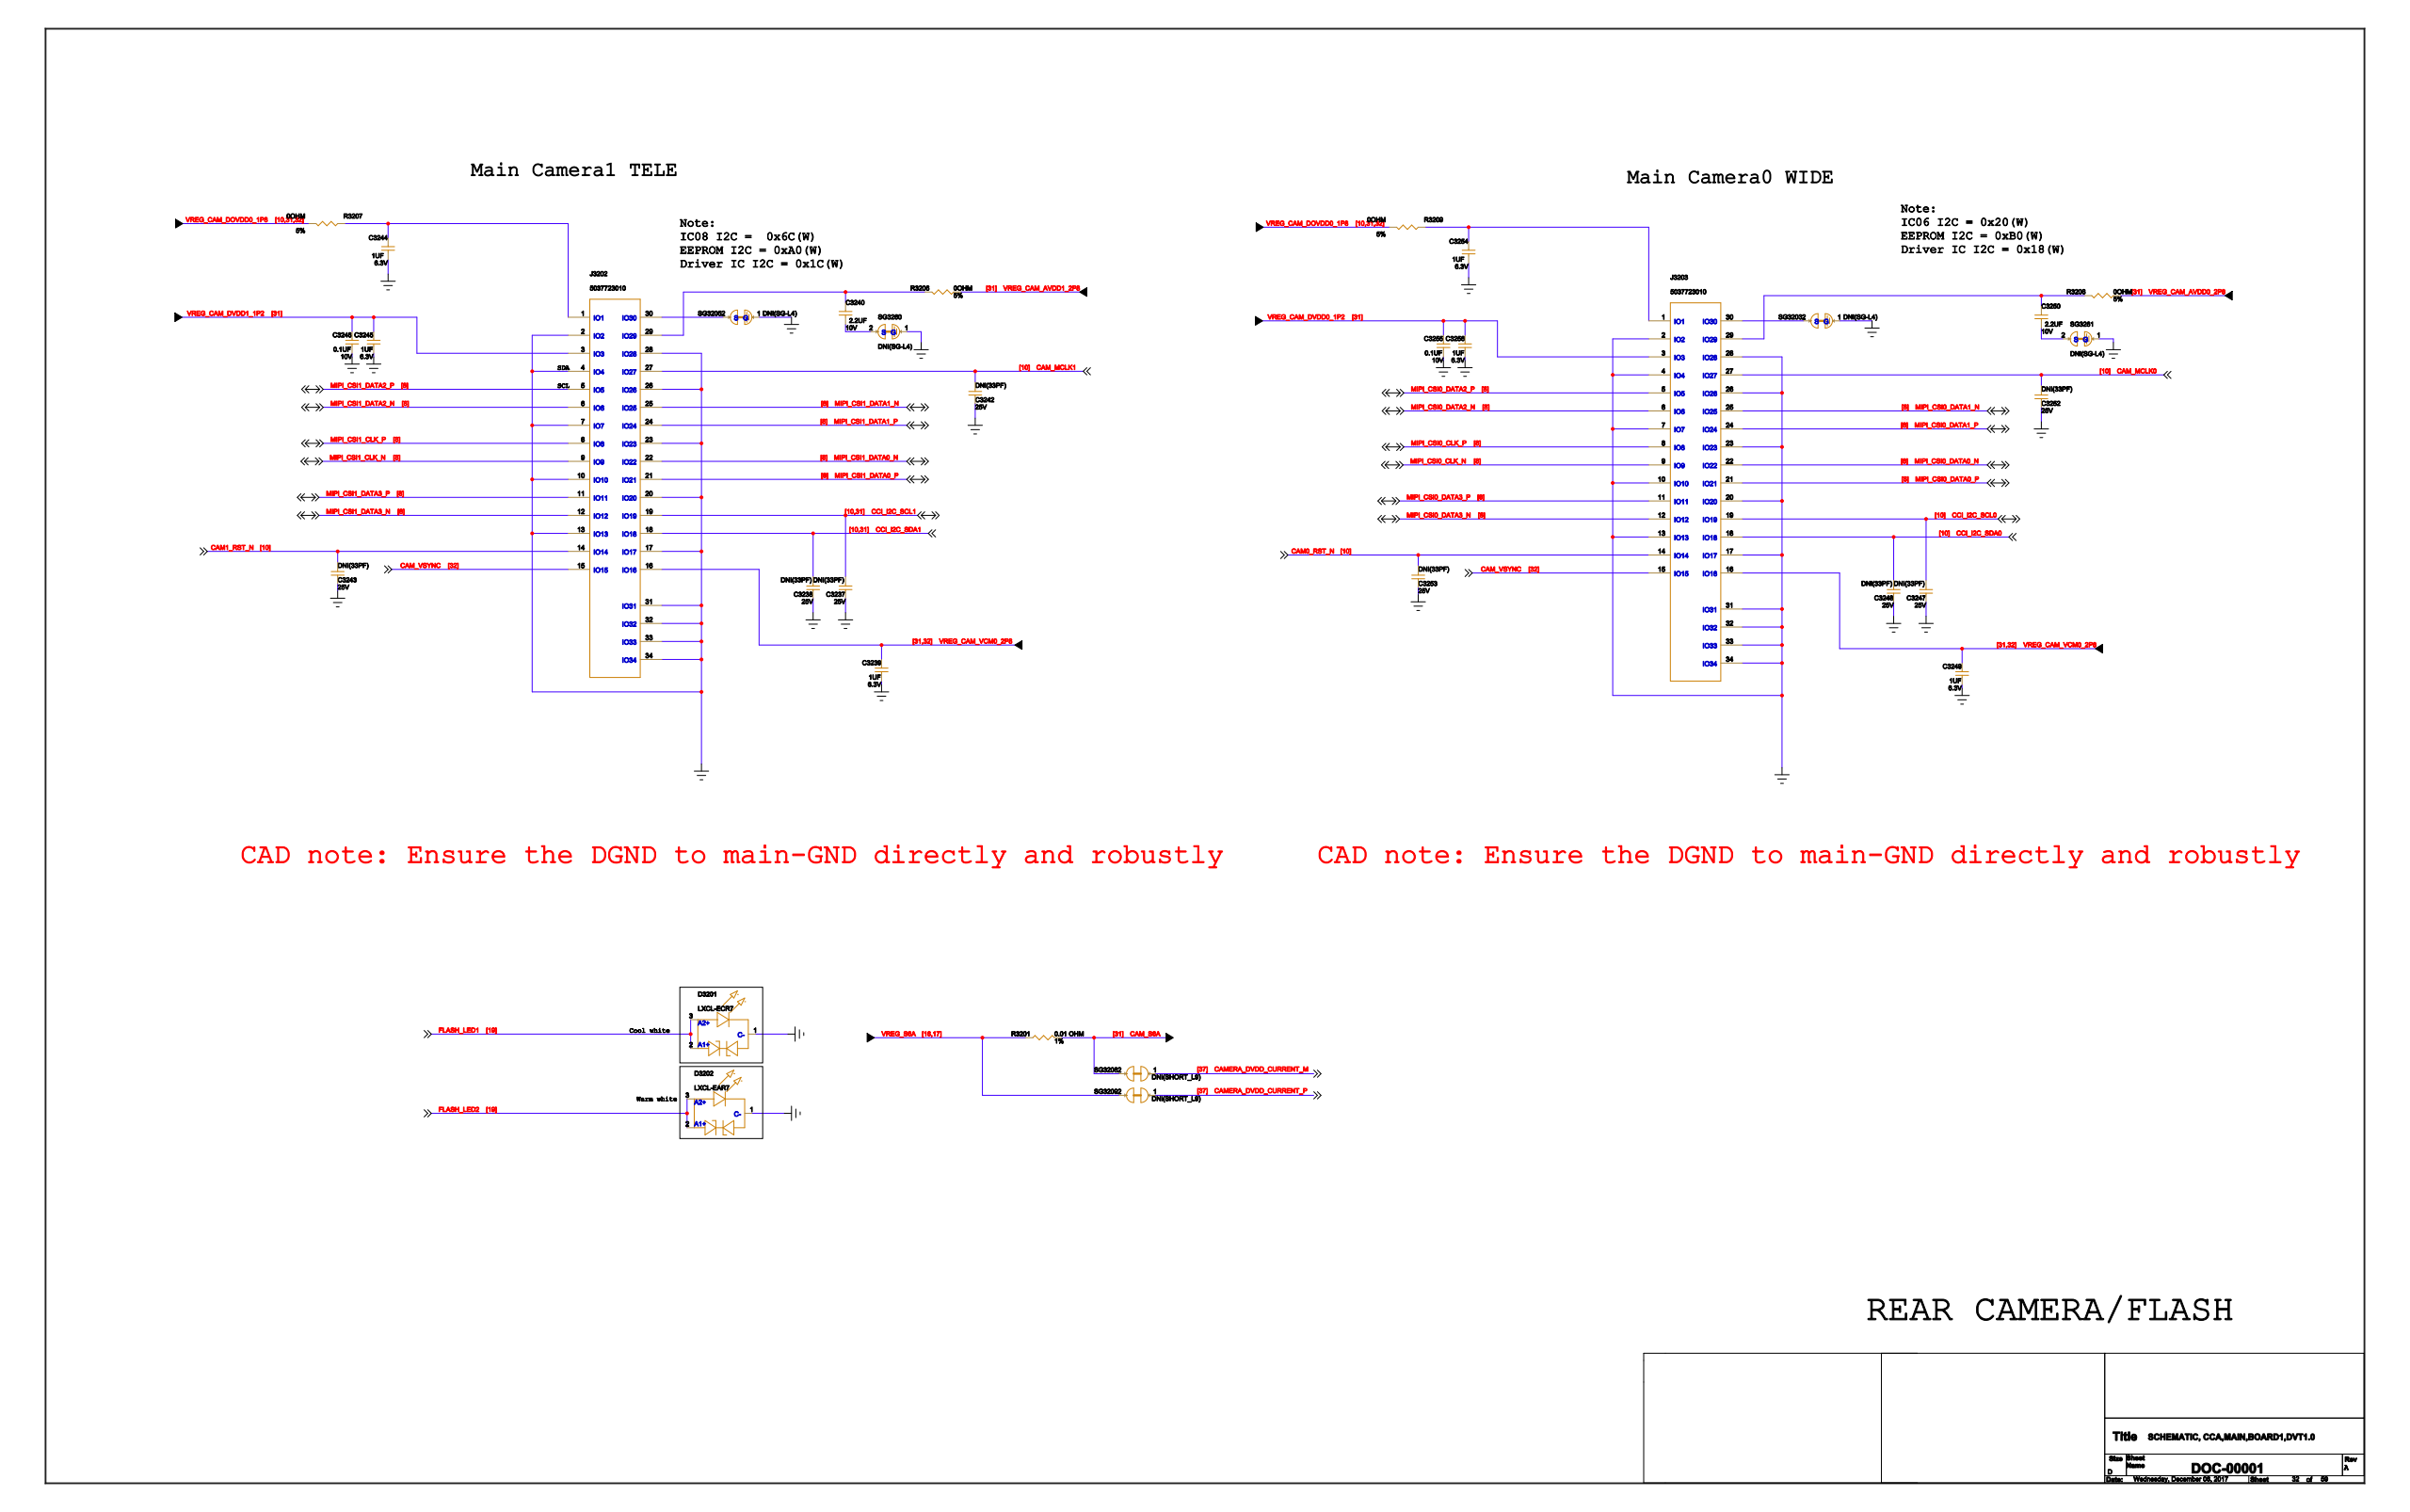Circuit board | KiCad | 1657 parts | 1365 nets | one sheet of the schematic
Parts on this sheet (reference | value | footprint):
C3237
C3238
C3239
C3240
C3242
C3243
C3244
C3245
C3246
C3247
C3248
C3249
C3250
C3252
C3253
C3254
C3255
C3256
D3202
J3202
J3203
R3201
R3206
R3207
R3208
R3209
SG3203
SG3205
SG3208
SG3209
SG3260
SG3261
Nets of these parts (net: part-pin ...):
GND: C3237-1 C3238-1 C3239-2 C3242-1 C3243-1 C3244-2 C3245-2 C3246-2 C3247-1 C3248-1 C3249-2 C3252-1 C3253-1 C3254-2 C3255-2 C3256-2 D3202-1 SG3203-1 SG3205-1 SG3260-1 SG3261-1 J3202-2 J3202-4 J3202-7 J3202-10 J3202-13 J3202-17 J3202-20 J3202-23 J3202-26 J3202-28 J3202-31 J3202-32 J3202-33 J3202-34 J3203-2 J3203-4 J3203-7 J3203-10 J3203-13 J3203-17 J3203-20 J3203-23 J3203-26 J3203-28 J3203-31 J3203-32 J3203-33 J3203-34
N21587930: SG3205-2 J3202-30
_CAM_DVDD1_1P2: C3245-1 C3246-1 J3202-3
N22393502: C3240-2 SG3260-2
_CAM_AVDD0_2P8: R3208-1
N21587625: C3250-1 R3208-2 J3203-29
N21587642: C3250-2 SG3261-2
CAM_DOVDD0_1P8: R3207-1 R3209-1
CCI_I2C_SCL0: C3247-2 J3203-19
_CAM_AVDD1_2P8: R3206-1
DVDD_CURRENT_P: SG3209-1
VREG_S6A: R3201-2 SG3209-2
CCI_I2C_SDA1: C3238-2 J3202-18
CAM_S6A: R3201-1 SG3208-2
N21588104: C3240-1 R3206-2 J3202-29
CCI_I2C_SCL1: C3237-2 J3202-19
CAM_MCLK1: C3242-2 J3202-27
_CAM_DVDD0_1P2: C3255-1 C3256-1 J3203-3
G_CAM_VCM0_2P8: C3239-1 C3249-1 J3202-16 J3203-16
CAM_MCLK0: C3252-2 J3203-27
N21587451: SG3203-2 J3203-30
CAM0_RST_N: C3253-2 J3203-14
CAM1_RST_N: C3243-2 J3202-14
CCI_I2C_SDA0: C3248-2 J3203-18
DVDD_CURRENT_M: SG3208-1
N21587772: C3244-1 R3207-2 J3202-1
CAM_VSYNC: J3202-15 J3203-15
N21587283: C3254-1 R3209-2 J3203-1
FLASH_LED2: D3202-2 D3202-3